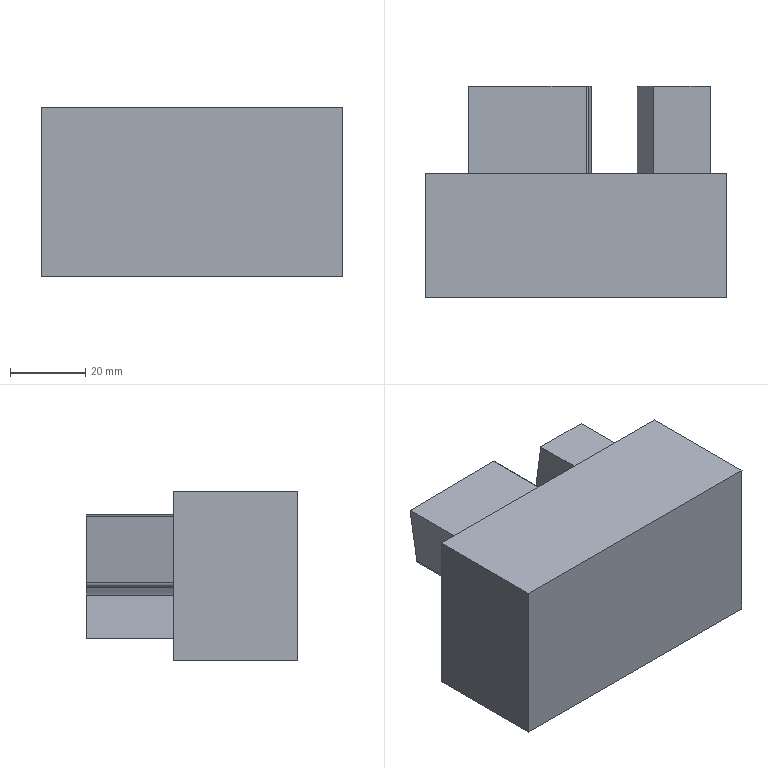Part | STEP file | 2004 | 1 solid | 29 faces | box 80 x 56 x 45 mm | volume 134107 mm3 | plane 23 | cylinder 5 | spline 1 | commonest cylinder face diameters 16.921 x2 2 x1 118.358 x1 497.751 x1